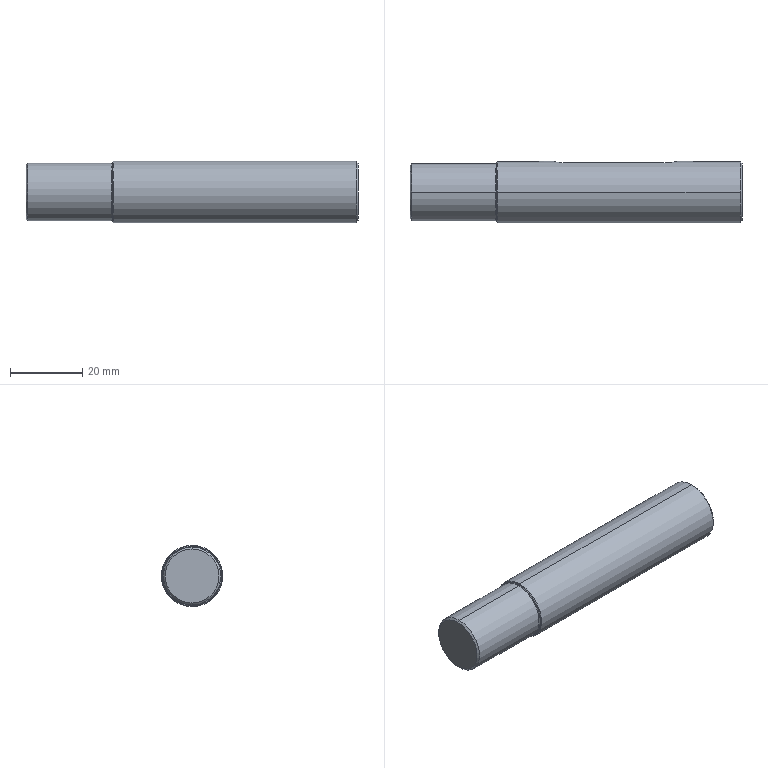Part | STEP file | 0245_003_PSFRF17-68.0-F24.0-P16-N5-KC16-A34 | 1 solid | 26 faces | box 92 x 17 x 17 mm | volume 19593 mm3 | cone 10 | cylinder 8 | plane 6 | torus 2 | commonest cylinder face diameters 4.2 x2 5 x2 16 x2 17 x2